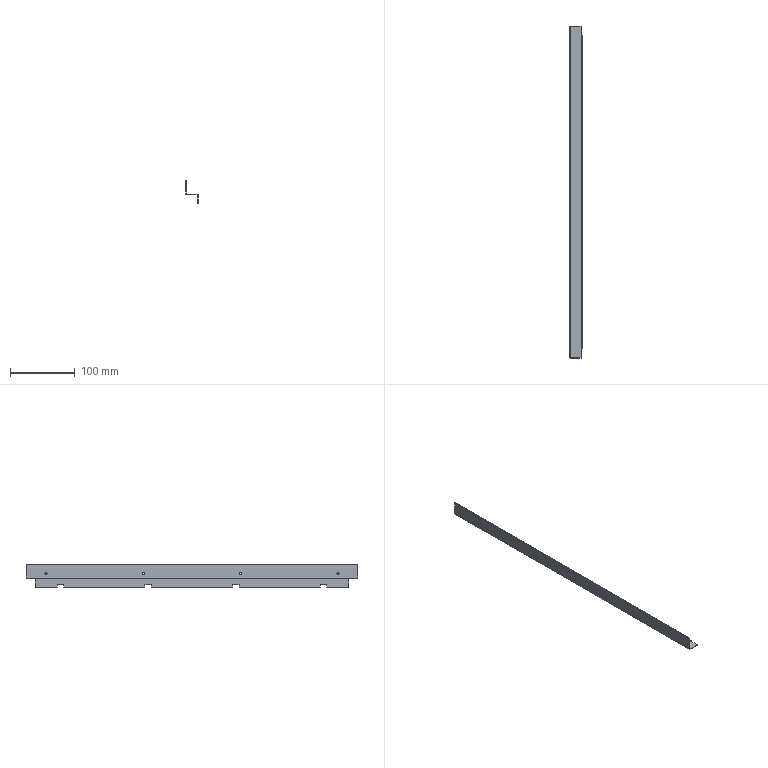Part | STEP file | 1 solid | 48 faces | box 18.5 x 511.5 x 34.7 mm | volume 20752 mm3 | plane 36 | cylinder 12 | commonest cylinder face diameters 3.3 x8 0.4 x2 2 x2